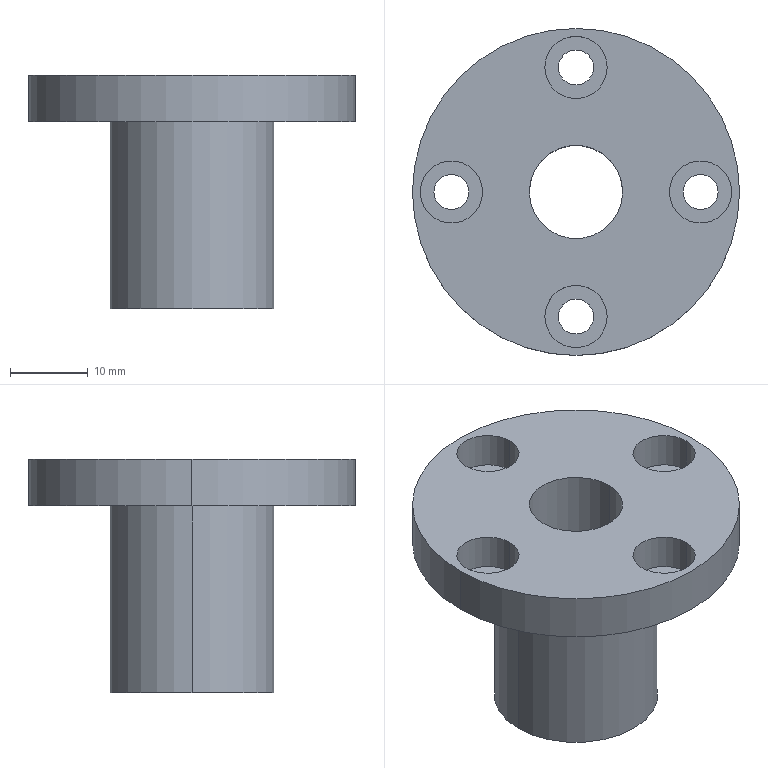Part | SolidWorks | features Extrusion 1, HoleWzd 1, ICE 1 | 1 solid | 29 faces | box 42 x 42 x 30 mm | volume 12218 mm3 | cylinder 22 | plane 7 | commonest cylinder face diameters 4.5 x8 8 x8 12 x2 21 x2 42 x2
STEP:
#1=CARTESIAN_POINT('',(-4.,16.,10.4));
#2=VERTEX_POINT('',#1);
#3=CARTESIAN_POINT('',(4.,16.,10.4));
#4=VERTEX_POINT('',#3);
#5=CARTESIAN_POINT('',(0.,16.,10.4));
#6=DIRECTION('',(0.,0.,1.));
#7=DIRECTION('',(1.,0.,0.));
#8=AXIS2_PLACEMENT_3D('',#5,#6,#7);
#9=CIRCLE('',#8,4.);
#10=EDGE_CURVE('',#2,#4,#9,.T.);
#11=ORIENTED_EDGE('',*,*,#10,.F.);
#12=CARTESIAN_POINT('',(-4.,16.,15.));
#13=VERTEX_POINT('',#12);
#14=CARTESIAN_POINT('',(-4.,16.,15.));
#15=DIRECTION('',(0.,0.,1.));
#16=VECTOR('',#15,1000.);
#17=LINE('',#14,#16);
#18=EDGE_CURVE('',#2,#13,#17,.T.);
#19=ORIENTED_EDGE('',*,*,#18,.T.);
#20=CARTESIAN_POINT('',(4.,16.,15.));
#21=VERTEX_POINT('',#20);
#22=CARTESIAN_POINT('',(0.,16.,15.));
#23=DIRECTION('',(0.,0.,1.));
#24=DIRECTION('',(1.,0.,0.));
#25=AXIS2_PLACEMENT_3D('',#22,#23,#24);
#26=CIRCLE('',#25,4.);
#27=EDGE_CURVE('',#13,#21,#26,.T.);
#28=ORIENTED_EDGE('',*,*,#27,.T.);
#29=CARTESIAN_POINT('',(4.,16.,15.));
#30=DIRECTION('',(0.,0.,1.));
#31=VECTOR('',#30,1000.);
#32=LINE('',#29,#31);
#33=EDGE_CURVE('',#4,#21,#32,.T.);
#34=ORIENTED_EDGE('',*,*,#33,.F.);
#35=EDGE_LOOP('',(#11,#19,#28,#34));
#36=FACE_OUTER_BOUND('',#35,.T.);
#37=CARTESIAN_POINT('',(0.,16.,15.));
#38=DIRECTION('',(0.,0.,1.));
#39=DIRECTION('',(1.,0.,0.));
#40=AXIS2_PLACEMENT_3D('',#37,#38,#39);
#41=CYLINDRICAL_SURFACE('',#40,4.);
#42=ADVANCED_FACE('',(#36),#41,.F.);
#43=CARTESIAN_POINT('',(-2.25,16.,9.));
#44=VERTEX_POINT('',#43);
#45=CARTESIAN_POINT('',(2.25,16.,9.));
#46=VERTEX_POINT('',#45);
#47=CARTESIAN_POINT('',(0.,16.,9.));
#48=DIRECTION('',(0.,0.,1.));
#49=DIRECTION('',(1.,0.,0.));
#50=AXIS2_PLACEMENT_3D('',#47,#48,#49);
#51=CIRCLE('',#50,2.25);
#52=EDGE_CURVE('',#44,#46,#51,.T.);
#53=ORIENTED_EDGE('',*,*,#52,.F.);
#54=CARTESIAN_POINT('',(-2.25,16.,10.4));
#55=VERTEX_POINT('',#54);
#56=CARTESIAN_POINT('',(-2.25,16.,15.));
#57=DIRECTION('',(0.,0.,1.));
#58=VECTOR('',#57,1000.);
#59=LINE('',#56,#58);
#60=EDGE_CURVE('',#44,#55,#59,.T.);
#61=ORIENTED_EDGE('',*,*,#60,.T.);
#62=CARTESIAN_POINT('',(2.25,16.,10.4));
#63=VERTEX_POINT('',#62);
#64=CARTESIAN_POINT('',(0.,16.,10.4));
#65=DIRECTION('',(0.,0.,1.));
#66=DIRECTION('',(1.,0.,0.));
#67=AXIS2_PLACEMENT_3D('',#64,#65,#66);
#68=CIRCLE('',#67,2.25);
#69=EDGE_CURVE('',#55,#63,#68,.T.);
#70=ORIENTED_EDGE('',*,*,#69,.T.);
#71=CARTESIAN_POINT('',(2.25,16.,15.));
#72=DIRECTION('',(0.,0.,1.));
#73=VECTOR('',#72,1000.);
#74=LINE('',#71,#73);
#75=EDGE_CURVE('',#46,#63,#74,.T.);
#76=ORIENTED_EDGE('',*,*,#75,.F.);
#77=EDGE_LOOP('',(#53,#61,#70,#76));
#78=FACE_OUTER_BOUND('',#77,.T.);
#79=CARTESIAN_POINT('',(0.,16.,15.));
#80=DIRECTION('',(0.,0.,1.));
#81=DIRECTION('',(1.,0.,0.));
#82=AXIS2_PLACEMENT_3D('',#79,#80,#81);
#83=CYLINDRICAL_SURFACE('',#82,2.25);
#84=ADVANCED_FACE('',(#78),#83,.F.);
#85=CARTESIAN_POINT('',(12.,0.,10.4));
#86=VERTEX_POINT('',#85);
#87=CARTESIAN_POINT('',(20.,0.,10.4));
#88=VERTEX_POINT('',#87);
#89=CARTESIAN_POINT('',(16.,0.,10.4));
#90=DIRECTION('',(0.,0.,1.));
#91=DIRECTION('',(1.,0.,0.));
#92=AXIS2_PLACEMENT_3D('',#89,#90,#91);
#93=CIRCLE('',#92,4.);
#94=EDGE_CURVE('',#86,#88,#93,.T.);
#95=ORIENTED_EDGE('',*,*,#94,.F.);
#96=CARTESIAN_POINT('',(12.,0.,15.));
#97=VERTEX_POINT('',#96);
#98=CARTESIAN_POINT('',(12.,0.,15.));
#99=DIRECTION('',(0.,0.,1.));
#100=VECTOR('',#99,1000.);
#101=LINE('',#98,#100);
#102=EDGE_CURVE('',#86,#97,#101,.T.);
#103=ORIENTED_EDGE('',*,*,#102,.T.);
#104=CARTESIAN_POINT('',(20.,0.,15.));
#105=VERTEX_POINT('',#104);
#106=CARTESIAN_POINT('',(16.,0.,15.));
#107=DIRECTION('',(0.,0.,1.));
#108=DIRECTION('',(1.,0.,0.));
#109=AXIS2_PLACEMENT_3D('',#106,#107,#108);
#110=CIRCLE('',#109,4.);
#111=EDGE_CURVE('',#97,#105,#110,.T.);
#112=ORIENTED_EDGE('',*,*,#111,.T.);
#113=CARTESIAN_POINT('',(20.,0.,15.));
#114=DIRECTION('',(0.,0.,1.));
#115=VECTOR('',#114,1000.);
#116=LINE('',#113,#115);
#117=EDGE_CURVE('',#88,#105,#116,.T.);
#118=ORIENTED_EDGE('',*,*,#117,.F.);
#119=EDGE_LOOP('',(#95,#103,#112,#118));
#120=FACE_OUTER_BOUND('',#119,.T.);
#121=CARTESIAN_POINT('',(16.,0.,15.));
#122=DIRECTION('',(0.,0.,1.));
#123=DIRECTION('',(1.,0.,0.));
#124=AXIS2_PLACEMENT_3D('',#121,#122,#123);
#125=CYLINDRICAL_SURFACE('',#124,4.);
#126=ADVANCED_FACE('',(#120),#125,.F.);
#127=CARTESIAN_POINT('',(13.75,0.,9.));
#128=VERTEX_POINT('',#127);
#129=CARTESIAN_POINT('',(18.25,0.,9.));
#130=VERTEX_POINT('',#129);
#131=CARTESIAN_POINT('',(16.,0.,9.));
#132=DIRECTION('',(0.,0.,1.));
#133=DIRECTION('',(1.,0.,0.));
#134=AXIS2_PLACEMENT_3D('',#131,#132,#133);
#135=CIRCLE('',#134,2.25);
#136=EDGE_CURVE('',#128,#130,#135,.T.);
#137=ORIENTED_EDGE('',*,*,#136,.F.);
#138=CARTESIAN_POINT('',(13.75,0.,10.4));
#139=VERTEX_POINT('',#138);
#140=CARTESIAN_POINT('',(13.75,0.,15.));
#141=DIRECTION('',(0.,0.,1.));
#142=VECTOR('',#141,1000.);
#143=LINE('',#140,#142);
#144=EDGE_CURVE('',#128,#139,#143,.T.);
#145=ORIENTED_EDGE('',*,*,#144,.T.);
#146=CARTESIAN_POINT('',(18.25,0.,10.4));
#147=VERTEX_POINT('',#146);
#148=CARTESIAN_POINT('',(16.,0.,10.4));
#149=DIRECTION('',(0.,0.,1.));
#150=DIRECTION('',(1.,0.,0.));
#151=AXIS2_PLACEMENT_3D('',#148,#149,#150);
#152=CIRCLE('',#151,2.25);
#153=EDGE_CURVE('',#139,#147,#152,.T.);
#154=ORIENTED_EDGE('',*,*,#153,.T.);
#155=CARTESIAN_POINT('',(18.25,0.,15.));
#156=DIRECTION('',(0.,0.,1.));
#157=VECTOR('',#156,1000.);
#158=LINE('',#155,#157);
#159=EDGE_CURVE('',#130,#147,#158,.T.);
#160=ORIENTED_EDGE('',*,*,#159,.F.);
#161=EDGE_LOOP('',(#137,#145,#154,#160));
#162=FACE_OUTER_BOUND('',#161,.T.);
#163=CARTESIAN_POINT('',(16.,0.,15.));
#164=DIRECTION('',(0.,0.,1.));
#165=DIRECTION('',(1.,0.,0.));
#166=AXIS2_PLACEMENT_3D('',#163,#164,#165);
#167=CYLINDRICAL_SURFACE('',#166,2.25);
#168=ADVANCED_FACE('',(#162),#167,.F.);
#169=CARTESIAN_POINT('',(-4.,-16.,10.4));
#170=VERTEX_POINT('',#169);
#171=CARTESIAN_POINT('',(4.,-16.,10.4));
#172=VERTEX_POINT('',#171);
#173=CARTESIAN_POINT('',(0.,-16.,10.4));
#174=DIRECTION('',(0.,0.,1.));
#175=DIRECTION('',(1.,0.,0.));
#176=AXIS2_PLACEMENT_3D('',#173,#174,#175);
#177=CIRCLE('',#176,4.);
#178=EDGE_CURVE('',#170,#172,#177,.T.);
#179=ORIENTED_EDGE('',*,*,#178,.F.);
#180=CARTESIAN_POINT('',(-4.,-16.,15.));
#181=VERTEX_POINT('',#180);
#182=CARTESIAN_POINT('',(-4.,-16.,15.));
#183=DIRECTION('',(0.,0.,1.));
#184=VECTOR('',#183,1000.);
#185=LINE('',#182,#184);
#186=EDGE_CURVE('',#170,#181,#185,.T.);
#187=ORIENTED_EDGE('',*,*,#186,.T.);
#188=CARTESIAN_POINT('',(4.,-16.,15.));
#189=VERTEX_POINT('',#188);
#190=CARTESIAN_POINT('',(0.,-16.,15.));
#191=DIRECTION('',(0.,0.,1.));
#192=DIRECTION('',(1.,0.,0.));
#193=AXIS2_PLACEMENT_3D('',#190,#191,#192);
#194=CIRCLE('',#193,4.);
#195=EDGE_CURVE('',#181,#189,#194,.T.);
#196=ORIENTED_EDGE('',*,*,#195,.T.);
#197=CARTESIAN_POINT('',(4.,-16.,15.));
#198=DIRECTION('',(0.,0.,1.));
#199=VECTOR('',#198,1000.);
#200=LINE('',#197,#199);
#201=EDGE_CURVE('',#172,#189,#200,.T.);
#202=ORIENTED_EDGE('',*,*,#201,.F.);
#203=EDGE_LOOP('',(#179,#187,#196,#202));
#204=FACE_OUTER_BOUND('',#203,.T.);
#205=CARTESIAN_POINT('',(0.,-16.,15.));
#206=DIRECTION('',(0.,0.,1.));
#207=DIRECTION('',(1.,0.,0.));
#208=AXIS2_PLACEMENT_3D('',#205,#206,#207);
#209=CYLINDRICAL_SURFACE('',#208,4.);
#210=ADVANCED_FACE('',(#204),#209,.F.);
#211=CARTESIAN_POINT('',(-2.25,-16.,9.));
#212=VERTEX_POINT('',#211);
#213=CARTESIAN_POINT('',(2.25,-16.,9.));
#214=VERTEX_POINT('',#213);
#215=CARTESIAN_POINT('',(0.,-16.,9.));
#216=DIRECTION('',(0.,0.,1.));
#217=DIRECTION('',(1.,0.,0.));
#218=AXIS2_PLACEMENT_3D('',#215,#216,#217);
#219=CIRCLE('',#218,2.25);
#220=EDGE_CURVE('',#212,#214,#219,.T.);
#221=ORIENTED_EDGE('',*,*,#220,.F.);
#222=CARTESIAN_POINT('',(-2.25,-16.,10.4));
#223=VERTEX_POINT('',#222);
#224=CARTESIAN_POINT('',(-2.25,-16.,15.));
#225=DIRECTION('',(0.,0.,1.));
#226=VECTOR('',#225,1000.);
#227=LINE('',#224,#226);
#228=EDGE_CURVE('',#212,#223,#227,.T.);
#229=ORIENTED_EDGE('',*,*,#228,.T.);
#230=CARTESIAN_POINT('',(2.25,-16.,10.4));
#231=VERTEX_POINT('',#230);
#232=CARTESIAN_POINT('',(0.,-16.,10.4));
#233=DIRECTION('',(0.,0.,1.));
#234=DIRECTION('',(1.,0.,0.));
#235=AXIS2_PLACEMENT_3D('',#232,#233,#234);
#236=CIRCLE('',#235,2.25);
#237=EDGE_CURVE('',#223,#231,#236,.T.);
#238=ORIENTED_EDGE('',*,*,#237,.T.);
#239=CARTESIAN_POINT('',(2.25,-16.,15.));
#240=DIRECTION('',(0.,0.,1.));
#241=VECTOR('',#240,1000.);
#242=LINE('',#239,#241);
#243=EDGE_CURVE('',#214,#231,#242,.T.);
#244=ORIENTED_EDGE('',*,*,#243,.F.);
#245=EDGE_LOOP('',(#221,#229,#238,#244));
#246=FACE_OUTER_BOUND('',#245,.T.);
#247=CARTESIAN_POINT('',(0.,-16.,15.));
#248=DIRECTION('',(0.,0.,1.));
#249=DIRECTION('',(1.,0.,0.));
#250=AXIS2_PLACEMENT_3D('',#247,#248,#249);
#251=CYLINDRICAL_SURFACE('',#250,2.25);
#252=ADVANCED_FACE('',(#246),#251,.F.);
#253=CARTESIAN_POINT('',(-20.,0.,10.4));
#254=VERTEX_POINT('',#253);
#255=CARTESIAN_POINT('',(-12.,0.,10.4));
#256=VERTEX_POINT('',#255);
#257=CARTESIAN_POINT('',(-16.,0.,10.4));
#258=DIRECTION('',(0.,0.,1.));
#259=DIRECTION('',(1.,0.,0.));
#260=AXIS2_PLACEMENT_3D('',#257,#258,#259);
#261=CIRCLE('',#260,4.);
#262=EDGE_CURVE('',#254,#256,#261,.T.);
#263=ORIENTED_EDGE('',*,*,#262,.F.);
#264=CARTESIAN_POINT('',(-20.,0.,15.));
#265=VERTEX_POINT('',#264);
#266=CARTESIAN_POINT('',(-20.,0.,15.));
#267=DIRECTION('',(0.,0.,1.));
#268=VECTOR('',#267,1000.);
#269=LINE('',#266,#268);
#270=EDGE_CURVE('',#254,#265,#269,.T.);
#271=ORIENTED_EDGE('',*,*,#270,.T.);
#272=CARTESIAN_POINT('',(-12.,0.,15.));
#273=VERTEX_POINT('',#272);
#274=CARTESIAN_POINT('',(-16.,0.,15.));
#275=DIRECTION('',(0.,0.,1.));
#276=DIRECTION('',(1.,0.,0.));
#277=AXIS2_PLACEMENT_3D('',#274,#275,#276);
#278=CIRCLE('',#277,4.);
#279=EDGE_CURVE('',#265,#273,#278,.T.);
#280=ORIENTED_EDGE('',*,*,#279,.T.);
#281=CARTESIAN_POINT('',(-12.,0.,15.));
#282=DIRECTION('',(0.,0.,1.));
#283=VECTOR('',#282,1000.);
#284=LINE('',#281,#283);
#285=EDGE_CURVE('',#256,#273,#284,.T.);
#286=ORIENTED_EDGE('',*,*,#285,.F.);
#287=EDGE_LOOP('',(#263,#271,#280,#286));
#288=FACE_OUTER_BOUND('',#287,.T.);
#289=CARTESIAN_POINT('',(-16.,0.,15.));
#290=DIRECTION('',(0.,0.,1.));
#291=DIRECTION('',(1.,0.,0.));
#292=AXIS2_PLACEMENT_3D('',#289,#290,#291);
#293=CYLINDRICAL_SURFACE('',#292,4.);
#294=ADVANCED_FACE('',(#288),#293,.F.);
#295=CARTESIAN_POINT('',(-18.25,0.,9.));
#296=VERTEX_POINT('',#295);
#297=CARTESIAN_POINT('',(-13.75,0.,9.));
#298=VERTEX_POINT('',#297);
#299=CARTESIAN_POINT('',(-16.,0.,9.));
#300=DIRECTION('',(0.,0.,1.));
#301=DIRECTION('',(1.,0.,0.));
#302=AXIS2_PLACEMENT_3D('',#299,#300,#301);
#303=CIRCLE('',#302,2.25);
#304=EDGE_CURVE('',#296,#298,#303,.T.);
#305=ORIENTED_EDGE('',*,*,#304,.F.);
#306=CARTESIAN_POINT('',(-18.25,0.,10.4));
#307=VERTEX_POINT('',#306);
#308=CARTESIAN_POINT('',(-18.25,0.,15.));
#309=DIRECTION('',(0.,0.,1.));
#310=VECTOR('',#309,1000.);
#311=LINE('',#308,#310);
#312=EDGE_CURVE('',#296,#307,#311,.T.);
#313=ORIENTED_EDGE('',*,*,#312,.T.);
#314=CARTESIAN_POINT('',(-13.75,0.,10.4));
#315=VERTEX_POINT('',#314);
#316=CARTESIAN_POINT('',(-16.,0.,10.4));
#317=DIRECTION('',(0.,0.,1.));
#318=DIRECTION('',(1.,0.,0.));
#319=AXIS2_PLACEMENT_3D('',#316,#317,#318);
#320=CIRCLE('',#319,2.25);
#321=EDGE_CURVE('',#307,#315,#320,.T.);
#322=ORIENTED_EDGE('',*,*,#321,.T.);
#323=CARTESIAN_POINT('',(-13.75,0.,15.));
#324=DIRECTION('',(0.,0.,1.));
#325=VECTOR('',#324,1000.);
#326=LINE('',#323,#325);
#327=EDGE_CURVE('',#298,#315,#326,.T.);
#328=ORIENTED_EDGE('',*,*,#327,.F.);
#329=EDGE_LOOP('',(#305,#313,#322,#328));
#330=FACE_OUTER_BOUND('',#329,.T.);
#331=CARTESIAN_POINT('',(-16.,0.,15.));
#332=DIRECTION('',(0.,0.,1.));
#333=DIRECTION('',(1.,0.,0.));
#334=AXIS2_PLACEMENT_3D('',#331,#332,#333);
#335=CYLINDRICAL_SURFACE('',#334,2.25);
#336=ADVANCED_FACE('',(#330),#335,.F.);
#337=CARTESIAN_POINT('',(21.,0.,9.));
#338=VERTEX_POINT('',#337);
#339=CARTESIAN_POINT('',(-21.,0.,9.));
#340=VERTEX_POINT('',#339);
#341=CARTESIAN_POINT('',(0.,0.,9.));
#342=DIRECTION('',(0.,0.,1.));
#343=DIRECTION('',(1.,0.,0.));
#344=AXIS2_PLACEMENT_3D('',#341,#342,#343);
#345=CIRCLE('',#344,21.);
#346=EDGE_CURVE('',#338,#340,#345,.T.);
#347=ORIENTED_EDGE('',*,*,#346,.T.);
#348=CARTESIAN_POINT('',(-21.,0.,15.));
#349=VERTEX_POINT('',#348);
#350=CARTESIAN_POINT('',(-21.,0.,9.));
#351=DIRECTION('',(0.,0.,1.));
#352=VECTOR('',#351,1000.);
#353=LINE('',#350,#352);
#354=EDGE_CURVE('',#340,#349,#353,.T.);
#355=ORIENTED_EDGE('',*,*,#354,.T.);
#356=CARTESIAN_POINT('',(21.,0.,15.));
#357=VERTEX_POINT('',#356);
#358=CARTESIAN_POINT('',(0.,0.,15.));
#359=DIRECTION('',(0.,0.,1.));
#360=DIRECTION('',(1.,0.,0.));
#361=AXIS2_PLACEMENT_3D('',#358,#359,#360);
#362=CIRCLE('',#361,21.);
#363=EDGE_CURVE('',#357,#349,#362,.T.);
#364=ORIENTED_EDGE('',*,*,#363,.F.);
#365=CARTESIAN_POINT('',(21.,0.,9.));
#366=DIRECTION('',(0.,0.,1.));
#367=VECTOR('',#366,1000.);
#368=LINE('',#365,#367);
#369=EDGE_CURVE('',#338,#357,#368,.T.);
#370=ORIENTED_EDGE('',*,*,#369,.F.);
#371=EDGE_LOOP('',(#347,#355,#364,#370));
#372=FACE_OUTER_BOUND('',#371,.T.);
#373=CARTESIAN_POINT('',(0.,0.,9.));
#374=DIRECTION('',(0.,0.,1.));
#375=DIRECTION('',(1.,0.,0.));
#376=AXIS2_PLACEMENT_3D('',#373,#374,#375);
#377=CYLINDRICAL_SURFACE('',#376,21.);
#378=ADVANCED_FACE('',(#372),#377,.T.);
#379=CARTESIAN_POINT('',(-6.,0.,15.));
#380=VERTEX_POINT('',#379);
#381=CARTESIAN_POINT('',(6.,0.,15.));
#382=VERTEX_POINT('',#381);
#383=CARTESIAN_POINT('',(0.,0.,15.));
#384=DIRECTION('',(0.,0.,1.));
#385=DIRECTION('',(1.,0.,0.));
#386=AXIS2_PLACEMENT_3D('',#383,#384,#385);
#387=CIRCLE('',#386,6.);
#388=EDGE_CURVE('',#380,#382,#387,.T.);
#389=ORIENTED_EDGE('',*,*,#388,.T.);
#390=CARTESIAN_POINT('',(6.,0.,-15.));
#391=VERTEX_POINT('',#390);
#392=CARTESIAN_POINT('',(6.,0.,15.));
#393=DIRECTION('',(0.,0.,-1.));
#394=VECTOR('',#393,1000.);
#395=LINE('',#392,#394);
#396=EDGE_CURVE('',#382,#391,#395,.T.);
#397=ORIENTED_EDGE('',*,*,#396,.T.);
#398=CARTESIAN_POINT('',(-6.,0.,-15.));
#399=VERTEX_POINT('',#398);
#400=CARTESIAN_POINT('',(0.,0.,-15.));
#401=DIRECTION('',(0.,0.,1.));
#402=DIRECTION('',(1.,0.,0.));
#403=AXIS2_PLACEMENT_3D('',#400,#401,#402);
#404=CIRCLE('',#403,6.);
#405=EDGE_CURVE('',#399,#391,#404,.T.);
#406=ORIENTED_EDGE('',*,*,#405,.F.);
#407=CARTESIAN_POINT('',(-6.,0.,15.));
#408=DIRECTION('',(0.,0.,-1.));
#409=VECTOR('',#408,1000.);
#410=LINE('',#407,#409);
#411=EDGE_CURVE('',#380,#399,#410,.T.);
#412=ORIENTED_EDGE('',*,*,#411,.F.);
#413=EDGE_LOOP('',(#389,#397,#406,#412));
#414=FACE_OUTER_BOUND('',#413,.T.);
#415=CARTESIAN_POINT('',(0.,0.,15.));
#416=DIRECTION('',(0.,0.,-1.));
#417=DIRECTION('',(-1.,0.,0.));
#418=AXIS2_PLACEMENT_3D('',#415,#416,#417);
#419=CYLINDRICAL_SURFACE('',#418,6.);
#420=ADVANCED_FACE('',(#414),#419,.F.);
#421=CARTESIAN_POINT('',(10.5,0.,9.));
#422=VERTEX_POINT('',#421);
#423=CARTESIAN_POINT('',(-10.5,0.,9.));
#424=VERTEX_POINT('',#423);
#425=CARTESIAN_POINT('',(0.,0.,9.));
#426=DIRECTION('',(0.,0.,1.));
#427=DIRECTION('',(1.,0.,0.));
#428=AXIS2_PLACEMENT_3D('',#425,#426,#427);
#429=CIRCLE('',#428,10.5);
#430=EDGE_CURVE('',#422,#424,#429,.T.);
#431=ORIENTED_EDGE('',*,*,#430,.F.);
#432=CARTESIAN_POINT('',(10.5,0.,-15.));
#433=VERTEX_POINT('',#432);
#434=CARTESIAN_POINT('',(10.5,0.,15.));
#435=DIRECTION('',(0.,0.,-1.));
#436=VECTOR('',#435,1000.);
#437=LINE('',#434,#436);
#438=EDGE_CURVE('',#422,#433,#437,.T.);
#439=ORIENTED_EDGE('',*,*,#438,.T.);
#440=CARTESIAN_POINT('',(-10.5,0.,-15.));
#441=VERTEX_POINT('',#440);
#442=CARTESIAN_POINT('',(0.,0.,-15.));
#443=DIRECTION('',(0.,0.,1.));
#444=DIRECTION('',(1.,0.,0.));
#445=AXIS2_PLACEMENT_3D('',#442,#443,#444);
#446=CIRCLE('',#445,10.5);
#447=EDGE_CURVE('',#433,#441,#446,.T.);
#448=ORIENTED_EDGE('',*,*,#447,.T.);
#449=CARTESIAN_POINT('',(-10.5,0.,15.));
#450=DIRECTION('',(0.,0.,-1.));
#451=VECTOR('',#450,1000.);
#452=LINE('',#449,#451);
#453=EDGE_CURVE('',#424,#441,#452,.T.);
#454=ORIENTED_EDGE('',*,*,#453,.F.);
#455=EDGE_LOOP('',(#431,#439,#448,#454));
#456=FACE_OUTER_BOUND('',#455,.T.);
#457=CARTESIAN_POINT('',(0.,0.,15.));
#458=DIRECTION('',(0.,0.,-1.));
#459=DIRECTION('',(-1.,0.,0.));
#460=AXIS2_PLACEMENT_3D('',#457,#458,#459);
#461=CYLINDRICAL_SURFACE('',#460,10.5);
#462=ADVANCED_FACE('',(#456),#461,.T.);
#463=ORIENTED_EDGE('',*,*,#438,.F.);
#464=CARTESIAN_POINT('',(0.,0.,9.));
#465=DIRECTION('',(0.,0.,1.));
#466=DIRECTION('',(1.,0.,0.));
#467=AXIS2_PLACEMENT_3D('',#464,#465,#466);
#468=CIRCLE('',#467,10.5);
#469=EDGE_CURVE('',#424,#422,#468,.T.);
#470=ORIENTED_EDGE('',*,*,#469,.F.);
#471=ORIENTED_EDGE('',*,*,#453,.T.);
#472=CARTESIAN_POINT('',(0.,0.,-15.));
#473=DIRECTION('',(0.,0.,1.));
#474=DIRECTION('',(1.,0.,0.));
#475=AXIS2_PLACEMENT_3D('',#472,#473,#474);
#476=CIRCLE('',#475,10.5);
#477=EDGE_CURVE('',#441,#433,#476,.T.);
#478=ORIENTED_EDGE('',*,*,#477,.T.);
#479=EDGE_LOOP('',(#463,#470,#471,#478));
#480=FACE_OUTER_BOUND('',#479,.T.);
#481=CARTESIAN_POINT('',(0.,0.,15.));
#482=DIRECTION('',(0.,0.,-1.));
#483=DIRECTION('',(-1.,0.,0.));
#484=AXIS2_PLACEMENT_3D('',#481,#482,#483);
#485=CYLINDRICAL_SURFACE('',#484,10.5);
#486=ADVANCED_FACE('',(#480),#485,.T.);
#487=CARTESIAN_POINT('',(0.,16.,15.));
#488=DIRECTION('',(0.,0.,1.));
#489=DIRECTION('',(1.,0.,0.));
#490=AXIS2_PLACEMENT_3D('',#487,#488,#489);
#491=CIRCLE('',#490,4.);
#492=EDGE_CURVE('',#21,#13,#491,.T.);
#493=ORIENTED_EDGE('',*,*,#492,.F.);
#494=ORIENTED_EDGE('',*,*,#27,.F.);
#495=EDGE_LOOP('',(#493,#494));
#496=FACE_BOUND('',#495,.T.);
#497=CARTESIAN_POINT('',(16.,0.,15.));
#498=DIRECTION('',(0.,0.,1.));
#499=DIRECTION('',(1.,0.,0.));
#500=AXIS2_PLACEMENT_3D('',#497,#498,#499);
#501=CIRCLE('',#500,4.);
#502=EDGE_CURVE('',#105,#97,#501,.T.);
#503=ORIENTED_EDGE('',*,*,#502,.F.);
#504=ORIENTED_EDGE('',*,*,#111,.F.);
#505=EDGE_LOOP('',(#503,#504));
#506=FACE_BOUND('',#505,.T.);
#507=CARTESIAN_POINT('',(0.,-16.,15.));
#508=DIRECTION('',(0.,0.,1.));
#509=DIRECTION('',(1.,0.,0.));
#510=AXIS2_PLACEMENT_3D('',#507,#508,#509);
#511=CIRCLE('',#510,4.);
#512=EDGE_CURVE('',#189,#181,#511,.T.);
#513=ORIENTED_EDGE('',*,*,#512,.F.);
#514=ORIENTED_EDGE('',*,*,#195,.F.);
#515=EDGE_LOOP('',(#513,#514));
#516=FACE_BOUND('',#515,.T.);
#517=CARTESIAN_POINT('',(-16.,0.,15.));
#518=DIRECTION('',(0.,0.,1.));
#519=DIRECTION('',(1.,0.,0.));
#520=AXIS2_PLACEMENT_3D('',#517,#518,#519);
#521=CIRCLE('',#520,4.);
#522=EDGE_CURVE('',#273,#265,#521,.T.);
#523=ORIENTED_EDGE('',*,*,#522,.F.);
#524=ORIENTED_EDGE('',*,*,#279,.F.);
#525=EDGE_LOOP('',(#523,#524));
#526=FACE_BOUND('',#525,.T.);
#527=ORIENTED_EDGE('',*,*,#388,.F.);
#528=CARTESIAN_POINT('',(0.,0.,15.));
#529=DIRECTION('',(0.,0.,1.));
#530=DIRECTION('',(1.,0.,0.));
#531=AXIS2_PLACEMENT_3D('',#528,#529,#530);
#532=CIRCLE('',#531,6.);
#533=EDGE_CURVE('',#382,#380,#532,.T.);
#534=ORIENTED_EDGE('',*,*,#533,.F.);
#535=EDGE_LOOP('',(#527,#534));
#536=FACE_BOUND('',#535,.T.);
#537=ORIENTED_EDGE('',*,*,#363,.T.);
#538=CARTESIAN_POINT('',(0.,0.,15.));
#539=DIRECTION('',(0.,0.,1.));
#540=DIRECTION('',(1.,0.,0.));
#541=AXIS2_PLACEMENT_3D('',#538,#539,#540);
#542=CIRCLE('',#541,21.);
#543=EDGE_CURVE('',#349,#357,#542,.T.);
#544=ORIENTED_EDGE('',*,*,#543,.T.);
#545=EDGE_LOOP('',(#537,#544));
#546=FACE_OUTER_BOUND('',#545,.T.);
#547=CARTESIAN_POINT('',(0.,0.,15.));
#548=DIRECTION('',(0.,0.,1.));
#549=DIRECTION('',(1.,0.,0.));
#550=AXIS2_PLACEMENT_3D('',#547,#548,#549);
#551=PLANE('',#550);
#552=ADVANCED_FACE('',(#496,#506,#516,#526,#536,#546),#551,.T.);
#553=ORIENTED_EDGE('',*,*,#477,.F.);
#554=ORIENTED_EDGE('',*,*,#447,.F.);
#555=EDGE_LOOP('',(#553,#554));
#556=FACE_OUTER_BOUND('',#555,.T.);
#557=ORIENTED_EDGE('',*,*,#405,.T.);
#558=CARTESIAN_POINT('',(0.,0.,-15.));
#559=DIRECTION('',(0.,0.,1.));
#560=DIRECTION('',(1.,0.,0.));
#561=AXIS2_PLACEMENT_3D('',#558,#559,#560);
#562=CIRCLE('',#561,6.);
#563=EDGE_CURVE('',#391,#399,#562,.T.);
#564=ORIENTED_EDGE('',*,*,#563,.T.);
#565=EDGE_LOOP('',(#557,#564));
#566=FACE_BOUND('',#565,.T.);
#567=CARTESIAN_POINT('',(0.,0.,-15.));
#568=DIRECTION('',(0.,0.,1.));
#569=DIRECTION('',(1.,0.,0.));
#570=AXIS2_PLACEMENT_3D('',#567,#568,#569);
#571=PLANE('',#570);
#572=ADVANCED_FACE('',(#556,#566),#571,.F.);
#573=ORIENTED_EDGE('',*,*,#396,.F.);
#574=ORIENTED_EDGE('',*,*,#533,.T.);
#575=ORIENTED_EDGE('',*,*,#411,.T.);
#576=ORIENTED_EDGE('',*,*,#563,.F.);
#577=EDGE_LOOP('',(#573,#574,#575,#576));
#578=FACE_OUTER_BOUND('',#577,.T.);
#579=CARTESIAN_POINT('',(0.,0.,15.));
#580=DIRECTION('',(0.,0.,-1.));
#581=DIRECTION('',(-1.,0.,0.));
#582=AXIS2_PLACEMENT_3D('',#579,#580,#581);
#583=CYLINDRICAL_SURFACE('',#582,6.);
#584=ADVANCED_FACE('',(#578),#583,.F.);
#585=ORIENTED_EDGE('',*,*,#354,.F.);
#586=CARTESIAN_POINT('',(0.,0.,9.));
#587=DIRECTION('',(0.,0.,1.));
#588=DIRECTION('',(1.,0.,0.));
#589=AXIS2_PLACEMENT_3D('',#586,#587,#588);
#590=CIRCLE('',#589,21.);
#591=EDGE_CURVE('',#340,#338,#590,.T.);
#592=ORIENTED_EDGE('',*,*,#591,.T.);
#593=ORIENTED_EDGE('',*,*,#369,.T.);
#594=ORIENTED_EDGE('',*,*,#543,.F.);
#595=EDGE_LOOP('',(#585,#592,#593,#594));
#596=FACE_OUTER_BOUND('',#595,.T.);
#597=CARTESIAN_POINT('',(0.,0.,9.));
#598=DIRECTION('',(0.,0.,1.));
#599=DIRECTION('',(1.,0.,0.));
#600=AXIS2_PLACEMENT_3D('',#597,#598,#599);
#601=CYLINDRICAL_SURFACE('',#600,21.);
#602=ADVANCED_FACE('',(#596),#601,.T.);
#603=CARTESIAN_POINT('',(0.,16.,9.));
#604=DIRECTION('',(0.,0.,1.));
#605=DIRECTION('',(1.,0.,0.));
#606=AXIS2_PLACEMENT_3D('',#603,#604,#605);
#607=CIRCLE('',#606,2.25);
#608=EDGE_CURVE('',#46,#44,#607,.T.);
#609=ORIENTED_EDGE('',*,*,#608,.T.);
#610=ORIENTED_EDGE('',*,*,#52,.T.);
#611=EDGE_LOOP('',(#609,#610));
#612=FACE_BOUND('',#611,.T.);
#613=CARTESIAN_POINT('',(16.,0.,9.));
#614=DIRECTION('',(0.,0.,1.));
#615=DIRECTION('',(1.,0.,0.));
#616=AXIS2_PLACEMENT_3D('',#613,#614,#615);
#617=CIRCLE('',#616,2.25);
#618=EDGE_CURVE('',#130,#128,#617,.T.);
#619=ORIENTED_EDGE('',*,*,#618,.T.);
#620=ORIENTED_EDGE('',*,*,#136,.T.);
#621=EDGE_LOOP('',(#619,#620));
#622=FACE_BOUND('',#621,.T.);
#623=CARTESIAN_POINT('',(0.,-16.,9.));
#624=DIRECTION('',(0.,0.,1.));
#625=DIRECTION('',(1.,0.,0.));
#626=AXIS2_PLACEMENT_3D('',#623,#624,#625);
#627=CIRCLE('',#626,2.25);
#628=EDGE_CURVE('',#214,#212,#627,.T.);
#629=ORIENTED_EDGE('',*,*,#628,.T.);
#630=ORIENTED_EDGE('',*,*,#220,.T.);
#631=EDGE_LOOP('',(#629,#630));
#632=FACE_BOUND('',#631,.T.);
#633=CARTESIAN_POINT('',(-16.,0.,9.));
#634=DIRECTION('',(0.,0.,1.));
#635=DIRECTION('',(1.,0.,0.));
#636=AXIS2_PLACEMENT_3D('',#633,#634,#635);
#637=CIRCLE('',#636,2.25);
#638=EDGE_CURVE('',#298,#296,#637,.T.);
#639=ORIENTED_EDGE('',*,*,#638,.T.);
#640=ORIENTED_EDGE('',*,*,#304,.T.);
#641=EDGE_LOOP('',(#639,#640));
#642=FACE_BOUND('',#641,.T.);
#643=ORIENTED_EDGE('',*,*,#469,.T.);
#644=ORIENTED_EDGE('',*,*,#430,.T.);
#645=EDGE_LOOP('',(#643,#644));
#646=FACE_BOUND('',#645,.T.);
#647=ORIENTED_EDGE('',*,*,#346,.F.);
#648=ORIENTED_EDGE('',*,*,#591,.F.);
#649=EDGE_LOOP('',(#647,#648));
#650=FACE_OUTER_BOUND('',#649,.T.);
#651=CARTESIAN_POINT('',(0.,0.,9.));
#652=DIRECTION('',(0.,0.,1.));
#653=DIRECTION('',(1.,0.,0.));
#654=AXIS2_PLACEMENT_3D('',#651,#652,#653);
#655=PLANE('',#654);
#656=ADVANCED_FACE('',(#612,#622,#632,#642,#646,#650),#655,.F.);
#657=ORIENTED_EDGE('',*,*,#312,.F.);
#658=ORIENTED_EDGE('',*,*,#638,.F.);
#659=ORIENTED_EDGE('',*,*,#327,.T.);
#660=CARTESIAN_POINT('',(-16.,0.,10.4));
#661=DIRECTION('',(0.,0.,1.));
#662=DIRECTION('',(1.,0.,0.));
#663=AXIS2_PLACEMENT_3D('',#660,#661,#662);
#664=CIRCLE('',#663,2.25);
#665=EDGE_CURVE('',#315,#307,#664,.T.);
#666=ORIENTED_EDGE('',*,*,#665,.T.);
#667=EDGE_LOOP('',(#657,#658,#659,#666));
#668=FACE_OUTER_BOUND('',#667,.T.);
#669=CARTESIAN_POINT('',(-16.,0.,15.));
#670=DIRECTION('',(0.,0.,1.));
#671=DIRECTION('',(1.,0.,0.));
#672=AXIS2_PLACEMENT_3D('',#669,#670,#671);
#673=CYLINDRICAL_SURFACE('',#672,2.25);
#674=ADVANCED_FACE('',(#668),#673,.F.);
#675=ORIENTED_EDGE('',*,*,#665,.F.);
#676=ORIENTED_EDGE('',*,*,#321,.F.);
#677=EDGE_LOOP('',(#675,#676));
#678=FACE_BOUND('',#677,.T.);
#679=CARTESIAN_POINT('',(-16.,0.,10.4));
#680=DIRECTION('',(0.,0.,1.));
#681=DIRECTION('',(1.,0.,0.));
#682=AXIS2_PLACEMENT_3D('',#679,#680,#681);
#683=CIRCLE('',#682,4.);
#684=EDGE_CURVE('',#256,#254,#683,.T.);
#685=ORIENTED_EDGE('',*,*,#684,.T.);
#686=ORIENTED_EDGE('',*,*,#262,.T.);
#687=EDGE_LOOP('',(#685,#686));
#688=FACE_OUTER_BOUND('',#687,.T.);
#689=CARTESIAN_POINT('',(-13.75,0.,10.4));
#690=DIRECTION('',(0.,0.,-1.));
#691=DIRECTION('',(-1.,0.,0.));
#692=AXIS2_PLACEMENT_3D('',#689,#690,#691);
#693=PLANE('',#692);
#694=ADVANCED_FACE('',(#678,#688),#693,.F.);
#695=ORIENTED_EDGE('',*,*,#270,.F.);
#696=ORIENTED_EDGE('',*,*,#684,.F.);
#697=ORIENTED_EDGE('',*,*,#285,.T.);
#698=ORIENTED_EDGE('',*,*,#522,.T.);
#699=EDGE_LOOP('',(#695,#696,#697,#698));
#700=FACE_OUTER_BOUND('',#699,.T.);
#701=CARTESIAN_POINT('',(-16.,0.,15.));
#702=DIRECTION('',(0.,0.,1.));
#703=DIRECTION('',(1.,0.,0.));
#704=AXIS2_PLACEMENT_3D('',#701,#702,#703);
#705=CYLINDRICAL_SURFACE('',#704,4.);
#706=ADVANCED_FACE('',(#700),#705,.F.);
#707=ORIENTED_EDGE('',*,*,#228,.F.);
#708=ORIENTED_EDGE('',*,*,#628,.F.);
#709=ORIENTED_EDGE('',*,*,#243,.T.);
#710=CARTESIAN_POINT('',(0.,-16.,10.4));
#711=DIRECTION('',(0.,0.,1.));
#712=DIRECTION('',(1.,0.,0.));
#713=AXIS2_PLACEMENT_3D('',#710,#711,#712);
#714=CIRCLE('',#713,2.25);
#715=EDGE_CURVE('',#231,#223,#714,.T.);
#716=ORIENTED_EDGE('',*,*,#715,.T.);
#717=EDGE_LOOP('',(#707,#708,#709,#716));
#718=FACE_OUTER_BOUND('',#717,.T.);
#719=CARTESIAN_POINT('',(0.,-16.,15.));
#720=DIRECTION('',(0.,0.,1.));
#721=DIRECTION('',(1.,0.,0.));
#722=AXIS2_PLACEMENT_3D('',#719,#720,#721);
#723=CYLINDRICAL_SURFACE('',#722,2.25);
#724=ADVANCED_FACE('',(#718),#723,.F.);
#725=ORIENTED_EDGE('',*,*,#715,.F.);
#726=ORIENTED_EDGE('',*,*,#237,.F.);
#727=EDGE_LOOP('',(#725,#726));
#728=FACE_BOUND('',#727,.T.);
#729=CARTESIAN_POINT('',(0.,-16.,10.4));
#730=DIRECTION('',(0.,0.,1.));
#731=DIRECTION('',(1.,0.,0.));
#732=AXIS2_PLACEMENT_3D('',#729,#730,#731);
#733=CIRCLE('',#732,4.);
#734=EDGE_CURVE('',#172,#170,#733,.T.);
#735=ORIENTED_EDGE('',*,*,#734,.T.);
#736=ORIENTED_EDGE('',*,*,#178,.T.);
#737=EDGE_LOOP('',(#735,#736));
#738=FACE_OUTER_BOUND('',#737,.T.);
#739=CARTESIAN_POINT('',(2.25,-16.,10.4));
#740=DIRECTION('',(0.,0.,-1.));
#741=DIRECTION('',(-1.,0.,0.));
#742=AXIS2_PLACEMENT_3D('',#739,#740,#741);
#743=PLANE('',#742);
#744=ADVANCED_FACE('',(#728,#738),#743,.F.);
#745=ORIENTED_EDGE('',*,*,#186,.F.);
#746=ORIENTED_EDGE('',*,*,#734,.F.);
#747=ORIENTED_EDGE('',*,*,#201,.T.);
#748=ORIENTED_EDGE('',*,*,#512,.T.);
#749=EDGE_LOOP('',(#745,#746,#747,#748));
#750=FACE_OUTER_BOUND('',#749,.T.);
#751=CARTESIAN_POINT('',(0.,-16.,15.));
#752=DIRECTION('',(0.,0.,1.));
#753=DIRECTION('',(1.,0.,0.));
#754=AXIS2_PLACEMENT_3D('',#751,#752,#753);
#755=CYLINDRICAL_SURFACE('',#754,4.);
#756=ADVANCED_FACE('',(#750),#755,.F.);
#757=ORIENTED_EDGE('',*,*,#144,.F.);
#758=ORIENTED_EDGE('',*,*,#618,.F.);
#759=ORIENTED_EDGE('',*,*,#159,.T.);
#760=CARTESIAN_POINT('',(16.,0.,10.4));
#761=DIRECTION('',(0.,0.,1.));
#762=DIRECTION('',(1.,0.,0.));
#763=AXIS2_PLACEMENT_3D('',#760,#761,#762);
#764=CIRCLE('',#763,2.25);
#765=EDGE_CURVE('',#147,#139,#764,.T.);
#766=ORIENTED_EDGE('',*,*,#765,.T.);
#767=EDGE_LOOP('',(#757,#758,#759,#766));
#768=FACE_OUTER_BOUND('',#767,.T.);
#769=CARTESIAN_POINT('',(16.,0.,15.));
#770=DIRECTION('',(0.,0.,1.));
#771=DIRECTION('',(1.,0.,0.));
#772=AXIS2_PLACEMENT_3D('',#769,#770,#771);
#773=CYLINDRICAL_SURFACE('',#772,2.25);
#774=ADVANCED_FACE('',(#768),#773,.F.);
#775=ORIENTED_EDGE('',*,*,#765,.F.);
#776=ORIENTED_EDGE('',*,*,#153,.F.);
#777=EDGE_LOOP('',(#775,#776));
#778=FACE_BOUND('',#777,.T.);
#779=CARTESIAN_POINT('',(16.,0.,10.4));
#780=DIRECTION('',(0.,0.,1.));
#781=DIRECTION('',(1.,0.,0.));
#782=AXIS2_PLACEMENT_3D('',#779,#780,#781);
#783=CIRCLE('',#782,4.);
#784=EDGE_CURVE('',#88,#86,#783,.T.);
#785=ORIENTED_EDGE('',*,*,#784,.T.);
#786=ORIENTED_EDGE('',*,*,#94,.T.);
#787=EDGE_LOOP('',(#785,#786));
#788=FACE_OUTER_BOUND('',#787,.T.);
#789=CARTESIAN_POINT('',(18.25,0.,10.4));
#790=DIRECTION('',(0.,0.,-1.));
#791=DIRECTION('',(-1.,0.,0.));
#792=AXIS2_PLACEMENT_3D('',#789,#790,#791);
#793=PLANE('',#792);
#794=ADVANCED_FACE('',(#778,#788),#793,.F.);
#795=ORIENTED_EDGE('',*,*,#102,.F.);
#796=ORIENTED_EDGE('',*,*,#784,.F.);
#797=ORIENTED_EDGE('',*,*,#117,.T.);
#798=ORIENTED_EDGE('',*,*,#502,.T.);
#799=EDGE_LOOP('',(#795,#796,#797,#798));
#800=FACE_OUTER_BOUND('',#799,.T.);
#801=CARTESIAN_POINT('',(16.,0.,15.));
#802=DIRECTION('',(0.,0.,1.));
#803=DIRECTION('',(1.,0.,0.));
#804=AXIS2_PLACEMENT_3D('',#801,#802,#803);
#805=CYLINDRICAL_SURFACE('',#804,4.);
#806=ADVANCED_FACE('',(#800),#805,.F.);
#807=ORIENTED_EDGE('',*,*,#60,.F.);
#808=ORIENTED_EDGE('',*,*,#608,.F.);
#809=ORIENTED_EDGE('',*,*,#75,.T.);
#810=CARTESIAN_POINT('',(0.,16.,10.4));
#811=DIRECTION('',(0.,0.,1.));
#812=DIRECTION('',(1.,0.,0.));
#813=AXIS2_PLACEMENT_3D('',#810,#811,#812);
#814=CIRCLE('',#813,2.25);
#815=EDGE_CURVE('',#63,#55,#814,.T.);
#816=ORIENTED_EDGE('',*,*,#815,.T.);
#817=EDGE_LOOP('',(#807,#808,#809,#816));
#818=FACE_OUTER_BOUND('',#817,.T.);
#819=CARTESIAN_POINT('',(0.,16.,15.));
#820=DIRECTION('',(0.,0.,1.));
#821=DIRECTION('',(1.,0.,0.));
#822=AXIS2_PLACEMENT_3D('',#819,#820,#821);
#823=CYLINDRICAL_SURFACE('',#822,2.25);
#824=ADVANCED_FACE('',(#818),#823,.F.);
#825=ORIENTED_EDGE('',*,*,#815,.F.);
#826=ORIENTED_EDGE('',*,*,#69,.F.);
#827=EDGE_LOOP('',(#825,#826));
#828=FACE_BOUND('',#827,.T.);
#829=CARTESIAN_POINT('',(0.,16.,10.4));
#830=DIRECTION('',(0.,0.,1.));
#831=DIRECTION('',(1.,0.,0.));
#832=AXIS2_PLACEMENT_3D('',#829,#830,#831);
#833=CIRCLE('',#832,4.);
#834=EDGE_CURVE('',#4,#2,#833,.T.);
#835=ORIENTED_EDGE('',*,*,#834,.T.);
#836=ORIENTED_EDGE('',*,*,#10,.T.);
#837=EDGE_LOOP('',(#835,#836));
#838=FACE_OUTER_BOUND('',#837,.T.);
#839=CARTESIAN_POINT('',(2.25,16.,10.4));
#840=DIRECTION('',(0.,0.,-1.));
#841=DIRECTION('',(-1.,0.,0.));
#842=AXIS2_PLACEMENT_3D('',#839,#840,#841);
#843=PLANE('',#842);
#844=ADVANCED_FACE('',(#828,#838),#843,.F.);
#845=ORIENTED_EDGE('',*,*,#18,.F.);
#846=ORIENTED_EDGE('',*,*,#834,.F.);
#847=ORIENTED_EDGE('',*,*,#33,.T.);
#848=ORIENTED_EDGE('',*,*,#492,.T.);
#849=EDGE_LOOP('',(#845,#846,#847,#848));
#850=FACE_OUTER_BOUND('',#849,.T.);
#851=CARTESIAN_POINT('',(0.,16.,15.));
#852=DIRECTION('',(0.,0.,1.));
#853=DIRECTION('',(1.,0.,0.));
#854=AXIS2_PLACEMENT_3D('',#851,#852,#853);
#855=CYLINDRICAL_SURFACE('',#854,4.);
#856=ADVANCED_FACE('',(#850),#855,.F.);
#857=CLOSED_SHELL('',(#42,#84,#126,#168,#210,#252,#294,#336,#378,#420,#462,#486,#552,#572,#584,#602,#656,#674,#694,#706,#724,#744,#756,#774,#794,#806,#824,#844,#856));
#858=MANIFOLD_SOLID_BREP('',#857);
#859=CARTESIAN_POINT('',(0.,0.,0.));
#860=DIRECTION('',(0.,0.,1.));
#861=DIRECTION('',(1.,0.,0.));
#862=AXIS2_PLACEMENT_3D('',#859,#860,#861);
#863=(LENGTH_UNIT()NAMED_UNIT(*)SI_UNIT(.MILLI.,.METRE.));
#864=UNCERTAINTY_MEASURE_WITH_UNIT(LENGTH_MEASURE(0.00001),#863,'','');
#865=(NAMED_UNIT(*)PLANE_ANGLE_UNIT()SI_UNIT($,.RADIAN.));
#866=(NAMED_UNIT(*)SI_UNIT($,.STERADIAN.)SOLID_ANGLE_UNIT());
#867=(GEOMETRIC_REPRESENTATION_CONTEXT(3)GLOBAL_UNCERTAINTY_ASSIGNED_CONTEXT((#864))GLOBAL_UNIT_ASSIGNED_CONTEXT((#863,#865,#866))REPRESENTATION_CONTEXT('',''));
#868=ADVANCED_BREP_SHAPE_REPRESENTATION('',(#858,#862),#867);